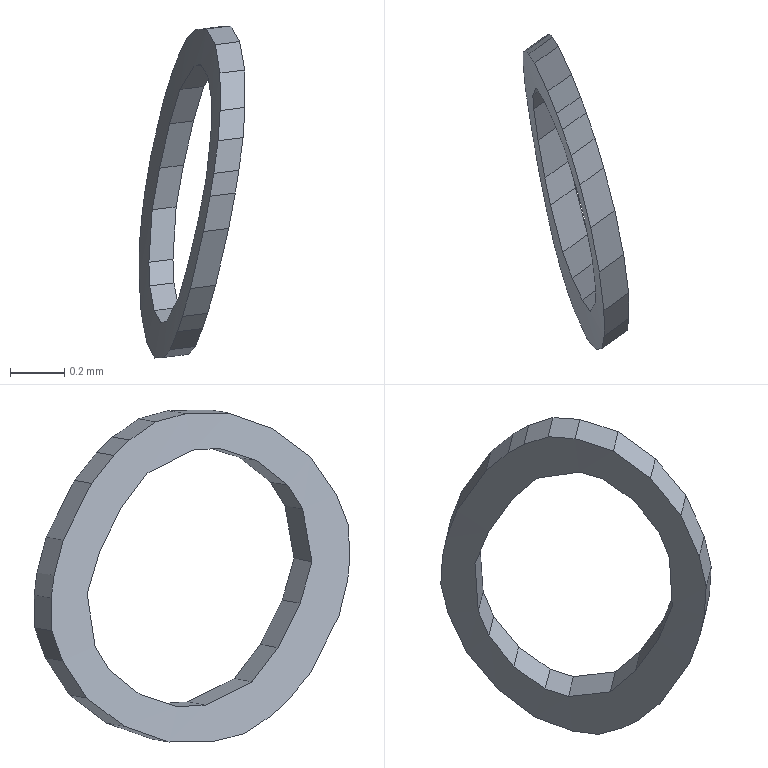Part | SolidWorks | features BaseBody 1 | 1 solid | 46 faces | box 0.3903 x 1.163 x 1.223 mm | volume 0.04564 mm3 | plane 44 | cylinder 2 | commonest cylinder face diameters 16.8 x1 17 x1